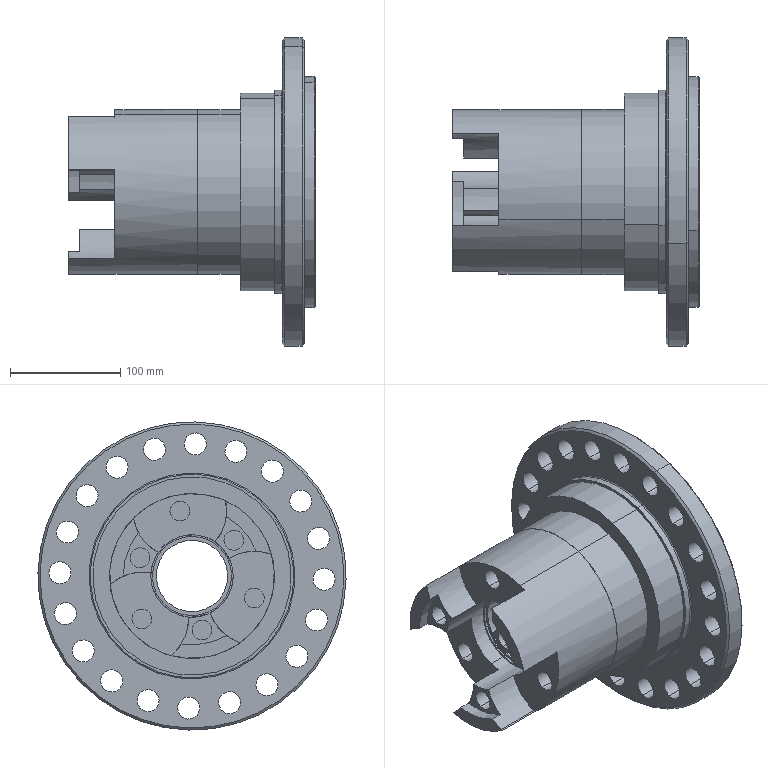Part | NX | features BREP 1 | 1 solid | 126 faces | box 224 x 280 x 280 mm | volume 3515315 mm3 | cylinder 89 | plane 27 | cone 8 | torus 2 | commonest cylinder face diameters 20 x40 18 x12 85 x8 72 x4 75 x4 125 x3